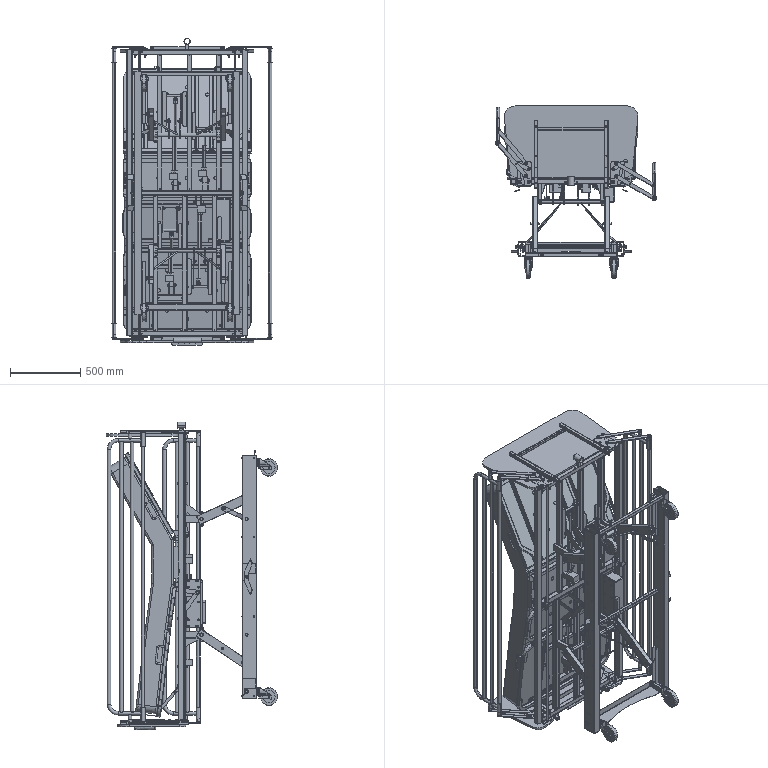Part | NX | features BREP 137 | 569 solids | 8387 faces | volume 292682019 mm3 | plane 3843 | cylinder 3536 | cone 724 | torus 176 | spline 74 | sphere 34 | commonest cylinder face diameters 3.175 x331 25.4 x213 9.525 x164 7.938 x160 12.7 x118 6.35 x116